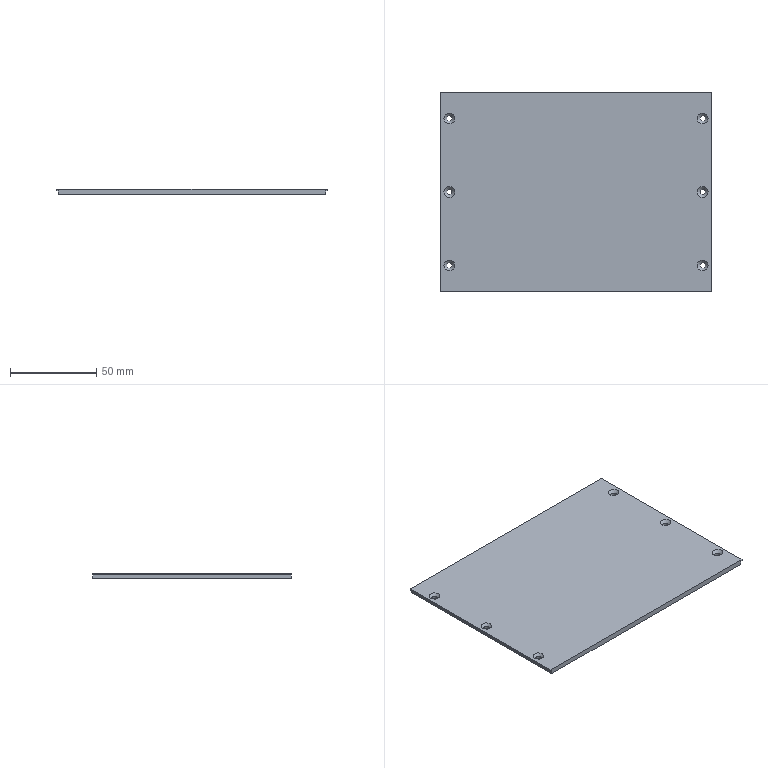Part | 1 solid | 50 faces | box 156.6 x 115 x 3 mm | volume 36735 mm3 | plane 26 | cylinder 18 | cone 6 | commonest cylinder face diameters 10 x12 3.2 x6
STEP:
#1=CARTESIAN_POINT('',(0.,115.,3.));
#2=VERTEX_POINT('',#1);
#3=CARTESIAN_POINT('',(0.,115.,2.1));
#4=VERTEX_POINT('',#3);
#5=CARTESIAN_POINT('',(0.,115.,3.));
#6=DIRECTION('',(0.,0.,-1.));
#7=VECTOR('',#6,1000.);
#8=LINE('',#5,#7);
#9=EDGE_CURVE('',#2,#4,#8,.T.);
#10=ORIENTED_EDGE('',*,*,#9,.T.);
#11=CARTESIAN_POINT('',(0.,0.,2.1));
#12=VERTEX_POINT('',#11);
#13=CARTESIAN_POINT('',(0.,-2.326,2.1));
#14=DIRECTION('',(0.,1.,0.));
#15=VECTOR('',#14,1000.);
#16=LINE('',#13,#15);
#17=EDGE_CURVE('',#12,#4,#16,.T.);
#18=ORIENTED_EDGE('',*,*,#17,.F.);
#19=CARTESIAN_POINT('',(0.,0.,3.));
#20=VERTEX_POINT('',#19);
#21=CARTESIAN_POINT('',(0.,0.,3.));
#22=DIRECTION('',(0.,0.,-1.));
#23=VECTOR('',#22,1000.);
#24=LINE('',#21,#23);
#25=EDGE_CURVE('',#20,#12,#24,.T.);
#26=ORIENTED_EDGE('',*,*,#25,.F.);
#27=CARTESIAN_POINT('',(0.,0.,3.));
#28=DIRECTION('',(0.,-1.,0.));
#29=VECTOR('',#28,1000.);
#30=LINE('',#27,#29);
#31=EDGE_CURVE('',#2,#20,#30,.T.);
#32=ORIENTED_EDGE('',*,*,#31,.F.);
#33=EDGE_LOOP('',(#10,#18,#26,#32));
#34=FACE_BOUND('',#33,.T.);
#35=CARTESIAN_POINT('',(0.,0.,3.));
#36=DIRECTION('',(1.,0.,0.));
#37=DIRECTION('',(0.,0.,-1.));
#38=AXIS2_PLACEMENT_3D('',#35,#36,#37);
#39=PLANE('',#38);
#40=ADVANCED_FACE('',(#34),#39,.F.);
#41=CARTESIAN_POINT('',(155.6,0.,2.1));
#42=VERTEX_POINT('',#41);
#43=CARTESIAN_POINT('',(155.6,0.,0.));
#44=VERTEX_POINT('',#43);
#45=CARTESIAN_POINT('',(155.6,0.,0.));
#46=DIRECTION('',(0.,0.,-1.));
#47=VECTOR('',#46,1000.);
#48=LINE('',#45,#47);
#49=EDGE_CURVE('',#42,#44,#48,.T.);
#50=ORIENTED_EDGE('',*,*,#49,.F.);
#51=CARTESIAN_POINT('',(156.6,0.,2.1));
#52=VERTEX_POINT('',#51);
#53=CARTESIAN_POINT('',(156.6,0.,2.1));
#54=DIRECTION('',(-1.,0.,0.));
#55=VECTOR('',#54,1000.);
#56=LINE('',#53,#55);
#57=EDGE_CURVE('',#52,#42,#56,.T.);
#58=ORIENTED_EDGE('',*,*,#57,.F.);
#59=CARTESIAN_POINT('',(156.6,0.,3.));
#60=VERTEX_POINT('',#59);
#61=CARTESIAN_POINT('',(156.6,0.,3.));
#62=DIRECTION('',(0.,0.,-1.));
#63=VECTOR('',#62,1000.);
#64=LINE('',#61,#63);
#65=EDGE_CURVE('',#60,#52,#64,.T.);
#66=ORIENTED_EDGE('',*,*,#65,.F.);
#67=CARTESIAN_POINT('',(0.,0.,3.));
#68=DIRECTION('',(1.,0.,0.));
#69=VECTOR('',#68,1000.);
#70=LINE('',#67,#69);
#71=EDGE_CURVE('',#20,#60,#70,.T.);
#72=ORIENTED_EDGE('',*,*,#71,.F.);
#73=ORIENTED_EDGE('',*,*,#25,.T.);
#74=CARTESIAN_POINT('',(1.,0.,2.1));
#75=VERTEX_POINT('',#74);
#76=CARTESIAN_POINT('',(0.,0.,2.1));
#77=DIRECTION('',(-1.,0.,0.));
#78=VECTOR('',#77,1000.);
#79=LINE('',#76,#78);
#80=EDGE_CURVE('',#75,#12,#79,.T.);
#81=ORIENTED_EDGE('',*,*,#80,.F.);
#82=CARTESIAN_POINT('',(1.,0.,0.));
#83=VERTEX_POINT('',#82);
#84=CARTESIAN_POINT('',(1.,0.,0.));
#85=DIRECTION('',(0.,0.,1.));
#86=VECTOR('',#85,1000.);
#87=LINE('',#84,#86);
#88=EDGE_CURVE('',#83,#75,#87,.T.);
#89=ORIENTED_EDGE('',*,*,#88,.F.);
#90=CARTESIAN_POINT('',(0.,0.,0.));
#91=DIRECTION('',(1.,0.,0.));
#92=VECTOR('',#91,1000.);
#93=LINE('',#90,#92);
#94=EDGE_CURVE('',#83,#44,#93,.T.);
#95=ORIENTED_EDGE('',*,*,#94,.T.);
#96=EDGE_LOOP('',(#50,#58,#66,#72,#73,#81,#89,#95));
#97=FACE_BOUND('',#96,.T.);
#98=CARTESIAN_POINT('',(0.,0.,3.));
#99=DIRECTION('',(0.,1.,0.));
#100=DIRECTION('',(0.,0.,1.));
#101=AXIS2_PLACEMENT_3D('',#98,#99,#100);
#102=PLANE('',#101);
#103=ADVANCED_FACE('',(#97),#102,.F.);
#104=ORIENTED_EDGE('',*,*,#65,.T.);
#105=CARTESIAN_POINT('',(156.6,115.,2.1));
#106=VERTEX_POINT('',#105);
#107=CARTESIAN_POINT('',(156.6,-2.326,2.1));
#108=DIRECTION('',(0.,1.,0.));
#109=VECTOR('',#108,1000.);
#110=LINE('',#107,#109);
#111=EDGE_CURVE('',#52,#106,#110,.T.);
#112=ORIENTED_EDGE('',*,*,#111,.T.);
#113=CARTESIAN_POINT('',(156.6,115.,3.));
#114=VERTEX_POINT('',#113);
#115=CARTESIAN_POINT('',(156.6,115.,3.));
#116=DIRECTION('',(0.,0.,-1.));
#117=VECTOR('',#116,1000.);
#118=LINE('',#115,#117);
#119=EDGE_CURVE('',#114,#106,#118,.T.);
#120=ORIENTED_EDGE('',*,*,#119,.F.);
#121=CARTESIAN_POINT('',(156.6,0.,3.));
#122=DIRECTION('',(0.,1.,0.));
#123=VECTOR('',#122,1000.);
#124=LINE('',#121,#123);
#125=EDGE_CURVE('',#60,#114,#124,.T.);
#126=ORIENTED_EDGE('',*,*,#125,.F.);
#127=EDGE_LOOP('',(#104,#112,#120,#126));
#128=FACE_BOUND('',#127,.T.);
#129=CARTESIAN_POINT('',(156.6,0.,3.));
#130=DIRECTION('',(-1.,0.,0.));
#131=DIRECTION('',(0.,0.,1.));
#132=AXIS2_PLACEMENT_3D('',#129,#130,#131);
#133=PLANE('',#132);
#134=ADVANCED_FACE('',(#128),#133,.F.);
#135=ORIENTED_EDGE('',*,*,#119,.T.);
#136=CARTESIAN_POINT('',(155.6,115.,2.1));
#137=VERTEX_POINT('',#136);
#138=CARTESIAN_POINT('',(156.6,115.,2.1));
#139=DIRECTION('',(1.,0.,0.));
#140=VECTOR('',#139,1000.);
#141=LINE('',#138,#140);
#142=EDGE_CURVE('',#137,#106,#141,.T.);
#143=ORIENTED_EDGE('',*,*,#142,.F.);
#144=CARTESIAN_POINT('',(155.6,115.,0.));
#145=VERTEX_POINT('',#144);
#146=CARTESIAN_POINT('',(155.6,115.,0.));
#147=DIRECTION('',(0.,0.,1.));
#148=VECTOR('',#147,1000.);
#149=LINE('',#146,#148);
#150=EDGE_CURVE('',#145,#137,#149,.T.);
#151=ORIENTED_EDGE('',*,*,#150,.F.);
#152=CARTESIAN_POINT('',(1.,115.,0.));
#153=VERTEX_POINT('',#152);
#154=CARTESIAN_POINT('',(0.,115.,0.));
#155=DIRECTION('',(-1.,0.,0.));
#156=VECTOR('',#155,1000.);
#157=LINE('',#154,#156);
#158=EDGE_CURVE('',#145,#153,#157,.T.);
#159=ORIENTED_EDGE('',*,*,#158,.T.);
#160=CARTESIAN_POINT('',(1.,115.,2.1));
#161=VERTEX_POINT('',#160);
#162=CARTESIAN_POINT('',(1.,115.,0.));
#163=DIRECTION('',(0.,0.,-1.));
#164=VECTOR('',#163,1000.);
#165=LINE('',#162,#164);
#166=EDGE_CURVE('',#161,#153,#165,.T.);
#167=ORIENTED_EDGE('',*,*,#166,.F.);
#168=CARTESIAN_POINT('',(0.,115.,2.1));
#169=DIRECTION('',(1.,0.,0.));
#170=VECTOR('',#169,1000.);
#171=LINE('',#168,#170);
#172=EDGE_CURVE('',#4,#161,#171,.T.);
#173=ORIENTED_EDGE('',*,*,#172,.F.);
#174=ORIENTED_EDGE('',*,*,#9,.F.);
#175=CARTESIAN_POINT('',(0.,115.,3.));
#176=DIRECTION('',(-1.,0.,0.));
#177=VECTOR('',#176,1000.);
#178=LINE('',#175,#177);
#179=EDGE_CURVE('',#114,#2,#178,.T.);
#180=ORIENTED_EDGE('',*,*,#179,.F.);
#181=EDGE_LOOP('',(#135,#143,#151,#159,#167,#173,#174,#180));
#182=FACE_BOUND('',#181,.T.);
#183=CARTESIAN_POINT('',(0.,115.,3.));
#184=DIRECTION('',(0.,-1.,0.));
#185=DIRECTION('',(0.,0.,-1.));
#186=AXIS2_PLACEMENT_3D('',#183,#184,#185);
#187=PLANE('',#186);
#188=ADVANCED_FACE('',(#182),#187,.F.);
#189=CARTESIAN_POINT('',(148.5,15.,3.));
#190=VERTEX_POINT('',#189);
#191=CARTESIAN_POINT('',(151.6,15.,3.));
#192=DIRECTION('',(0.,0.,-1.));
#193=DIRECTION('',(-1.,0.,0.));
#194=AXIS2_PLACEMENT_3D('',#191,#192,#193);
#195=CIRCLE('',#194,3.1);
#196=EDGE_CURVE('',#190,#190,#195,.T.);
#197=ORIENTED_EDGE('',*,*,#196,.T.);
#198=EDGE_LOOP('',(#197));
#199=FACE_BOUND('',#198,.T.);
#200=CARTESIAN_POINT('',(148.5,57.5,3.));
#201=VERTEX_POINT('',#200);
#202=CARTESIAN_POINT('',(151.6,57.5,3.));
#203=DIRECTION('',(0.,0.,-1.));
#204=DIRECTION('',(-1.,0.,0.));
#205=AXIS2_PLACEMENT_3D('',#202,#203,#204);
#206=CIRCLE('',#205,3.1);
#207=EDGE_CURVE('',#201,#201,#206,.T.);
#208=ORIENTED_EDGE('',*,*,#207,.T.);
#209=EDGE_LOOP('',(#208));
#210=FACE_BOUND('',#209,.T.);
#211=CARTESIAN_POINT('',(148.5,100.,3.));
#212=VERTEX_POINT('',#211);
#213=CARTESIAN_POINT('',(151.6,100.,3.));
#214=DIRECTION('',(0.,0.,-1.));
#215=DIRECTION('',(-1.,0.,0.));
#216=AXIS2_PLACEMENT_3D('',#213,#214,#215);
#217=CIRCLE('',#216,3.1);
#218=EDGE_CURVE('',#212,#212,#217,.T.);
#219=ORIENTED_EDGE('',*,*,#218,.T.);
#220=EDGE_LOOP('',(#219));
#221=FACE_BOUND('',#220,.T.);
#222=CARTESIAN_POINT('',(1.9,15.,3.));
#223=VERTEX_POINT('',#222);
#224=CARTESIAN_POINT('',(5.,15.,3.));
#225=DIRECTION('',(0.,0.,-1.));
#226=DIRECTION('',(-1.,0.,0.));
#227=AXIS2_PLACEMENT_3D('',#224,#225,#226);
#228=CIRCLE('',#227,3.1);
#229=EDGE_CURVE('',#223,#223,#228,.T.);
#230=ORIENTED_EDGE('',*,*,#229,.T.);
#231=EDGE_LOOP('',(#230));
#232=FACE_BOUND('',#231,.T.);
#233=CARTESIAN_POINT('',(1.9,57.5,3.));
#234=VERTEX_POINT('',#233);
#235=CARTESIAN_POINT('',(5.,57.5,3.));
#236=DIRECTION('',(0.,0.,-1.));
#237=DIRECTION('',(-1.,0.,0.));
#238=AXIS2_PLACEMENT_3D('',#235,#236,#237);
#239=CIRCLE('',#238,3.1);
#240=EDGE_CURVE('',#234,#234,#239,.T.);
#241=ORIENTED_EDGE('',*,*,#240,.T.);
#242=EDGE_LOOP('',(#241));
#243=FACE_BOUND('',#242,.T.);
#244=CARTESIAN_POINT('',(1.9,100.,3.));
#245=VERTEX_POINT('',#244);
#246=CARTESIAN_POINT('',(5.,100.,3.));
#247=DIRECTION('',(0.,0.,-1.));
#248=DIRECTION('',(-1.,0.,0.));
#249=AXIS2_PLACEMENT_3D('',#246,#247,#248);
#250=CIRCLE('',#249,3.1);
#251=EDGE_CURVE('',#245,#245,#250,.T.);
#252=ORIENTED_EDGE('',*,*,#251,.T.);
#253=EDGE_LOOP('',(#252));
#254=FACE_BOUND('',#253,.T.);
#255=ORIENTED_EDGE('',*,*,#31,.T.);
#256=ORIENTED_EDGE('',*,*,#71,.T.);
#257=ORIENTED_EDGE('',*,*,#125,.T.);
#258=ORIENTED_EDGE('',*,*,#179,.T.);
#259=EDGE_LOOP('',(#255,#256,#257,#258));
#260=FACE_BOUND('',#259,.T.);
#261=CARTESIAN_POINT('',(0.,0.,3.));
#262=DIRECTION('',(0.,0.,-1.));
#263=DIRECTION('',(-1.,0.,0.));
#264=AXIS2_PLACEMENT_3D('',#261,#262,#263);
#265=PLANE('',#264);
#266=ADVANCED_FACE('',(#199,#210,#221,#232,#243,#254,#260),#265,.F.);
#267=CARTESIAN_POINT('',(81.083,52.031,0.));
#268=VERTEX_POINT('',#267);
#269=CARTESIAN_POINT('',(130.154,19.154,0.));
#270=VERTEX_POINT('',#269);
#271=CARTESIAN_POINT('',(78.3,53.896,0.));
#272=DIRECTION('',(0.8308,-0.5566,0.));
#273=VECTOR('',#272,1000.);
#274=LINE('',#271,#273);
#275=EDGE_CURVE('',#268,#270,#274,.T.);
#276=ORIENTED_EDGE('',*,*,#275,.F.);
#277=CARTESIAN_POINT('',(75.517,52.031,0.));
#278=VERTEX_POINT('',#277);
#279=CARTESIAN_POINT('',(78.3,47.878,0.));
#280=DIRECTION('',(0.,0.,-1.));
#281=DIRECTION('',(-1.,0.,0.));
#282=AXIS2_PLACEMENT_3D('',#279,#280,#281);
#283=CIRCLE('',#282,5.);
#284=EDGE_CURVE('',#268,#278,#283,.F.);
#285=ORIENTED_EDGE('',*,*,#284,.T.);
#286=CARTESIAN_POINT('',(26.446,19.154,0.));
#287=VERTEX_POINT('',#286);
#288=CARTESIAN_POINT('',(78.3,53.896,0.));
#289=DIRECTION('',(0.8308,0.5566,0.));
#290=VECTOR('',#289,1000.);
#291=LINE('',#288,#290);
#292=EDGE_CURVE('',#287,#278,#291,.T.);
#293=ORIENTED_EDGE('',*,*,#292,.F.);
#294=CARTESIAN_POINT('',(29.229,10.,0.));
#295=VERTEX_POINT('',#294);
#296=CARTESIAN_POINT('',(29.229,15.,0.));
#297=DIRECTION('',(0.,0.,-1.));
#298=DIRECTION('',(-1.,0.,0.));
#299=AXIS2_PLACEMENT_3D('',#296,#297,#298);
#300=CIRCLE('',#299,5.);
#301=EDGE_CURVE('',#287,#295,#300,.F.);
#302=ORIENTED_EDGE('',*,*,#301,.T.);
#303=CARTESIAN_POINT('',(127.371,10.,0.));
#304=VERTEX_POINT('',#303);
#305=CARTESIAN_POINT('',(143.817,10.,0.));
#306=DIRECTION('',(-1.,0.,0.));
#307=VECTOR('',#306,1000.);
#308=LINE('',#305,#307);
#309=EDGE_CURVE('',#304,#295,#308,.T.);
#310=ORIENTED_EDGE('',*,*,#309,.F.);
#311=CARTESIAN_POINT('',(127.371,15.,0.));
#312=DIRECTION('',(0.,0.,-1.));
#313=DIRECTION('',(-1.,0.,0.));
#314=AXIS2_PLACEMENT_3D('',#311,#312,#313);
#315=CIRCLE('',#314,5.);
#316=EDGE_CURVE('',#304,#270,#315,.F.);
#317=ORIENTED_EDGE('',*,*,#316,.T.);
#318=EDGE_LOOP('',(#276,#285,#293,#302,#310,#317));
#319=FACE_BOUND('',#318,.T.);
#320=CARTESIAN_POINT('',(10.,23.522,0.));
#321=VERTEX_POINT('',#320);
#322=CARTESIAN_POINT('',(10.,91.478,0.));
#323=VERTEX_POINT('',#322);
#324=CARTESIAN_POINT('',(10.,14.154,0.));
#325=DIRECTION('',(0.,1.,0.));
#326=VECTOR('',#325,1000.);
#327=LINE('',#324,#326);
#328=EDGE_CURVE('',#321,#323,#327,.T.);
#329=ORIENTED_EDGE('',*,*,#328,.F.);
#330=CARTESIAN_POINT('',(17.783,19.368,0.));
#331=VERTEX_POINT('',#330);
#332=CARTESIAN_POINT('',(15.,23.522,0.));
#333=DIRECTION('',(0.,0.,-1.));
#334=DIRECTION('',(-1.,0.,0.));
#335=AXIS2_PLACEMENT_3D('',#332,#333,#334);
#336=CIRCLE('',#335,5.);
#337=EDGE_CURVE('',#321,#331,#336,.F.);
#338=ORIENTED_EDGE('',*,*,#337,.T.);
#339=CARTESIAN_POINT('',(68.496,53.346,0.));
#340=VERTEX_POINT('',#339);
#341=CARTESIAN_POINT('',(10.,14.154,0.));
#342=DIRECTION('',(-0.8308,-0.5566,0.));
#343=VECTOR('',#342,1000.);
#344=LINE('',#341,#343);
#345=EDGE_CURVE('',#340,#331,#344,.T.);
#346=ORIENTED_EDGE('',*,*,#345,.F.);
#347=CARTESIAN_POINT('',(68.496,61.654,0.));
#348=VERTEX_POINT('',#347);
#349=CARTESIAN_POINT('',(65.713,57.5,0.));
#350=DIRECTION('',(0.,0.,-1.));
#351=DIRECTION('',(-1.,0.,0.));
#352=AXIS2_PLACEMENT_3D('',#349,#350,#351);
#353=CIRCLE('',#352,5.);
#354=EDGE_CURVE('',#340,#348,#353,.F.);
#355=ORIENTED_EDGE('',*,*,#354,.T.);
#356=CARTESIAN_POINT('',(17.783,95.632,0.));
#357=VERTEX_POINT('',#356);
#358=CARTESIAN_POINT('',(10.,100.846,0.));
#359=DIRECTION('',(0.8308,-0.5566,0.));
#360=VECTOR('',#359,1000.);
#361=LINE('',#358,#360);
#362=EDGE_CURVE('',#357,#348,#361,.T.);
#363=ORIENTED_EDGE('',*,*,#362,.F.);
#364=CARTESIAN_POINT('',(15.,91.478,0.));
#365=DIRECTION('',(0.,0.,-1.));
#366=DIRECTION('',(-1.,0.,0.));
#367=AXIS2_PLACEMENT_3D('',#364,#365,#366);
#368=CIRCLE('',#367,5.);
#369=EDGE_CURVE('',#357,#323,#368,.F.);
#370=ORIENTED_EDGE('',*,*,#369,.T.);
#371=EDGE_LOOP('',(#329,#338,#346,#355,#363,#370));
#372=FACE_BOUND('',#371,.T.);
#373=CARTESIAN_POINT('',(75.517,62.969,0.));
#374=VERTEX_POINT('',#373);
#375=CARTESIAN_POINT('',(26.446,95.846,0.));
#376=VERTEX_POINT('',#375);
#377=CARTESIAN_POINT('',(78.3,61.104,0.));
#378=DIRECTION('',(-0.8308,0.5566,0.));
#379=VECTOR('',#378,1000.);
#380=LINE('',#377,#379);
#381=EDGE_CURVE('',#374,#376,#380,.T.);
#382=ORIENTED_EDGE('',*,*,#381,.F.);
#383=CARTESIAN_POINT('',(81.083,62.969,0.));
#384=VERTEX_POINT('',#383);
#385=CARTESIAN_POINT('',(78.3,67.122,0.));
#386=DIRECTION('',(0.,0.,-1.));
#387=DIRECTION('',(-1.,0.,0.));
#388=AXIS2_PLACEMENT_3D('',#385,#386,#387);
#389=CIRCLE('',#388,5.);
#390=EDGE_CURVE('',#374,#384,#389,.F.);
#391=ORIENTED_EDGE('',*,*,#390,.T.);
#392=CARTESIAN_POINT('',(130.154,95.846,0.));
#393=VERTEX_POINT('',#392);
#394=CARTESIAN_POINT('',(78.3,61.104,0.));
#395=DIRECTION('',(-0.8308,-0.5566,0.));
#396=VECTOR('',#395,1000.);
#397=LINE('',#394,#396);
#398=EDGE_CURVE('',#393,#384,#397,.T.);
#399=ORIENTED_EDGE('',*,*,#398,.F.);
#400=CARTESIAN_POINT('',(127.371,105.,0.));
#401=VERTEX_POINT('',#400);
#402=CARTESIAN_POINT('',(127.371,100.,0.));
#403=DIRECTION('',(0.,0.,-1.));
#404=DIRECTION('',(-1.,0.,0.));
#405=AXIS2_PLACEMENT_3D('',#402,#403,#404);
#406=CIRCLE('',#405,5.);
#407=EDGE_CURVE('',#393,#401,#406,.F.);
#408=ORIENTED_EDGE('',*,*,#407,.T.);
#409=CARTESIAN_POINT('',(29.229,105.,0.));
#410=VERTEX_POINT('',#409);
#411=CARTESIAN_POINT('',(143.817,105.,0.));
#412=DIRECTION('',(1.,0.,0.));
#413=VECTOR('',#412,1000.);
#414=LINE('',#411,#413);
#415=EDGE_CURVE('',#410,#401,#414,.T.);
#416=ORIENTED_EDGE('',*,*,#415,.F.);
#417=CARTESIAN_POINT('',(29.229,100.,0.));
#418=DIRECTION('',(0.,0.,-1.));
#419=DIRECTION('',(-1.,0.,0.));
#420=AXIS2_PLACEMENT_3D('',#417,#418,#419);
#421=CIRCLE('',#420,5.);
#422=EDGE_CURVE('',#410,#376,#421,.F.);
#423=ORIENTED_EDGE('',*,*,#422,.T.);
#424=EDGE_LOOP('',(#382,#391,#399,#408,#416,#423));
#425=FACE_BOUND('',#424,.T.);
#426=CARTESIAN_POINT('',(88.104,61.654,0.));
#427=VERTEX_POINT('',#426);
#428=CARTESIAN_POINT('',(138.817,95.632,0.));
#429=VERTEX_POINT('',#428);
#430=CARTESIAN_POINT('',(146.6,100.846,0.));
#431=DIRECTION('',(0.8308,0.5566,0.));
#432=VECTOR('',#431,1000.);
#433=LINE('',#430,#432);
#434=EDGE_CURVE('',#427,#429,#433,.T.);
#435=ORIENTED_EDGE('',*,*,#434,.F.);
#436=CARTESIAN_POINT('',(88.104,53.346,0.));
#437=VERTEX_POINT('',#436);
#438=CARTESIAN_POINT('',(90.887,57.5,0.));
#439=DIRECTION('',(0.,0.,-1.));
#440=DIRECTION('',(-1.,0.,0.));
#441=AXIS2_PLACEMENT_3D('',#438,#439,#440);
#442=CIRCLE('',#441,5.);
#443=EDGE_CURVE('',#427,#437,#442,.F.);
#444=ORIENTED_EDGE('',*,*,#443,.T.);
#445=CARTESIAN_POINT('',(138.817,19.368,0.));
#446=VERTEX_POINT('',#445);
#447=CARTESIAN_POINT('',(146.6,14.154,0.));
#448=DIRECTION('',(-0.8308,0.5566,0.));
#449=VECTOR('',#448,1000.);
#450=LINE('',#447,#449);
#451=EDGE_CURVE('',#446,#437,#450,.T.);
#452=ORIENTED_EDGE('',*,*,#451,.F.);
#453=CARTESIAN_POINT('',(146.6,23.522,0.));
#454=VERTEX_POINT('',#453);
#455=CARTESIAN_POINT('',(141.6,23.522,0.));
#456=DIRECTION('',(0.,0.,-1.));
#457=DIRECTION('',(-1.,0.,0.));
#458=AXIS2_PLACEMENT_3D('',#455,#456,#457);
#459=CIRCLE('',#458,5.);
#460=EDGE_CURVE('',#446,#454,#459,.F.);
#461=ORIENTED_EDGE('',*,*,#460,.T.);
#462=CARTESIAN_POINT('',(146.6,91.478,0.));
#463=VERTEX_POINT('',#462);
#464=CARTESIAN_POINT('',(146.6,14.154,0.));
#465=DIRECTION('',(0.,-1.,0.));
#466=VECTOR('',#465,1000.);
#467=LINE('',#464,#466);
#468=EDGE_CURVE('',#463,#454,#467,.T.);
#469=ORIENTED_EDGE('',*,*,#468,.F.);
#470=CARTESIAN_POINT('',(141.6,91.478,0.));
#471=DIRECTION('',(0.,0.,-1.));
#472=DIRECTION('',(-1.,0.,0.));
#473=AXIS2_PLACEMENT_3D('',#470,#471,#472);
#474=CIRCLE('',#473,5.);
#475=EDGE_CURVE('',#463,#429,#474,.F.);
#476=ORIENTED_EDGE('',*,*,#475,.T.);
#477=EDGE_LOOP('',(#435,#444,#452,#461,#469,#476));
#478=FACE_BOUND('',#477,.T.);
#479=CARTESIAN_POINT('',(155.6,-2.326,0.));
#480=DIRECTION('',(0.,1.,0.));
#481=VECTOR('',#480,1000.);
#482=LINE('',#479,#481);
#483=EDGE_CURVE('',#44,#145,#482,.T.);
#484=ORIENTED_EDGE('',*,*,#483,.F.);
#485=ORIENTED_EDGE('',*,*,#94,.F.);
#486=CARTESIAN_POINT('',(1.,-2.326,0.));
#487=DIRECTION('',(0.,1.,0.));
#488=VECTOR('',#487,1000.);
#489=LINE('',#486,#488);
#490=EDGE_CURVE('',#83,#153,#489,.T.);
#491=ORIENTED_EDGE('',*,*,#490,.T.);
#492=ORIENTED_EDGE('',*,*,#158,.F.);
#493=EDGE_LOOP('',(#484,#485,#491,#492));
#494=FACE_BOUND('',#493,.T.);
#495=CARTESIAN_POINT('',(150.,100.,0.));
#496=VERTEX_POINT('',#495);
#497=CARTESIAN_POINT('',(151.6,100.,0.));
#498=DIRECTION('',(0.,0.,-1.));
#499=DIRECTION('',(-1.,0.,0.));
#500=AXIS2_PLACEMENT_3D('',#497,#498,#499);
#501=CIRCLE('',#500,1.6);
#502=EDGE_CURVE('',#496,#496,#501,.F.);
#503=ORIENTED_EDGE('',*,*,#502,.T.);
#504=EDGE_LOOP('',(#503));
#505=FACE_BOUND('',#504,.T.);
#506=CARTESIAN_POINT('',(150.,57.5,0.));
#507=VERTEX_POINT('',#506);
#508=CARTESIAN_POINT('',(151.6,57.5,0.));
#509=DIRECTION('',(0.,0.,-1.));
#510=DIRECTION('',(-1.,0.,0.));
#511=AXIS2_PLACEMENT_3D('',#508,#509,#510);
#512=CIRCLE('',#511,1.6);
#513=EDGE_CURVE('',#507,#507,#512,.F.);
#514=ORIENTED_EDGE('',*,*,#513,.T.);
#515=EDGE_LOOP('',(#514));
#516=FACE_BOUND('',#515,.T.);
#517=CARTESIAN_POINT('',(150.,15.,0.));
#518=VERTEX_POINT('',#517);
#519=CARTESIAN_POINT('',(151.6,15.,0.));
#520=DIRECTION('',(0.,0.,-1.));
#521=DIRECTION('',(-1.,0.,0.));
#522=AXIS2_PLACEMENT_3D('',#519,#520,#521);
#523=CIRCLE('',#522,1.6);
#524=EDGE_CURVE('',#518,#518,#523,.F.);
#525=ORIENTED_EDGE('',*,*,#524,.T.);
#526=EDGE_LOOP('',(#525));
#527=FACE_BOUND('',#526,.T.);
#528=CARTESIAN_POINT('',(3.4,15.,0.));
#529=VERTEX_POINT('',#528);
#530=CARTESIAN_POINT('',(5.,15.,0.));
#531=DIRECTION('',(0.,0.,-1.));
#532=DIRECTION('',(-1.,0.,0.));
#533=AXIS2_PLACEMENT_3D('',#530,#531,#532);
#534=CIRCLE('',#533,1.6);
#535=EDGE_CURVE('',#529,#529,#534,.F.);
#536=ORIENTED_EDGE('',*,*,#535,.T.);
#537=EDGE_LOOP('',(#536));
#538=FACE_BOUND('',#537,.T.);
#539=CARTESIAN_POINT('',(3.4,57.5,0.));
#540=VERTEX_POINT('',#539);
#541=CARTESIAN_POINT('',(5.,57.5,0.));
#542=DIRECTION('',(0.,0.,-1.));
#543=DIRECTION('',(-1.,0.,0.));
#544=AXIS2_PLACEMENT_3D('',#541,#542,#543);
#545=CIRCLE('',#544,1.6);
#546=EDGE_CURVE('',#540,#540,#545,.F.);
#547=ORIENTED_EDGE('',*,*,#546,.T.);
#548=EDGE_LOOP('',(#547));
#549=FACE_BOUND('',#548,.T.);
#550=CARTESIAN_POINT('',(3.4,100.,0.));
#551=VERTEX_POINT('',#550);
#552=CARTESIAN_POINT('',(5.,100.,0.));
#553=DIRECTION('',(0.,0.,-1.));
#554=DIRECTION('',(-1.,0.,0.));
#555=AXIS2_PLACEMENT_3D('',#552,#553,#554);
#556=CIRCLE('',#555,1.6);
#557=EDGE_CURVE('',#551,#551,#556,.F.);
#558=ORIENTED_EDGE('',*,*,#557,.T.);
#559=EDGE_LOOP('',(#558));
#560=FACE_BOUND('',#559,.T.);
#561=CARTESIAN_POINT('',(0.,0.,0.));
#562=DIRECTION('',(0.,0.,-1.));
#563=DIRECTION('',(-1.,0.,0.));
#564=AXIS2_PLACEMENT_3D('',#561,#562,#563);
#565=PLANE('',#564);
#566=ADVANCED_FACE('',(#319,#372,#425,#478,#494,#505,#516,#527,#538,#549,#560),#565,.T.);
#567=CARTESIAN_POINT('',(3.4,100.,1.5));
#568=VERTEX_POINT('',#567);
#569=CARTESIAN_POINT('',(5.,100.,1.5));
#570=DIRECTION('',(0.,0.,-1.));
#571=DIRECTION('',(-1.,0.,0.));
#572=AXIS2_PLACEMENT_3D('',#569,#570,#571);
#573=CIRCLE('',#572,1.6);
#574=EDGE_CURVE('',#568,#568,#573,.F.);
#575=ORIENTED_EDGE('',*,*,#574,.T.);
#576=EDGE_LOOP('',(#575));
#577=FACE_BOUND('',#576,.T.);
#578=ORIENTED_EDGE('',*,*,#557,.F.);
#579=EDGE_LOOP('',(#578));
#580=FACE_BOUND('',#579,.T.);
#581=CARTESIAN_POINT('',(5.,100.,-4.525));
#582=DIRECTION('',(0.,0.,1.));
#583=DIRECTION('',(1.,0.,0.));
#584=AXIS2_PLACEMENT_3D('',#581,#582,#583);
#585=CYLINDRICAL_SURFACE('',#584,1.6);
#586=ADVANCED_FACE('',(#577,#580),#585,.F.);
#587=CARTESIAN_POINT('',(3.4,57.5,1.5));
#588=VERTEX_POINT('',#587);
#589=CARTESIAN_POINT('',(5.,57.5,1.5));
#590=DIRECTION('',(0.,0.,-1.));
#591=DIRECTION('',(-1.,0.,0.));
#592=AXIS2_PLACEMENT_3D('',#589,#590,#591);
#593=CIRCLE('',#592,1.6);
#594=EDGE_CURVE('',#588,#588,#593,.F.);
#595=ORIENTED_EDGE('',*,*,#594,.T.);
#596=EDGE_LOOP('',(#595));
#597=FACE_BOUND('',#596,.T.);
#598=ORIENTED_EDGE('',*,*,#546,.F.);
#599=EDGE_LOOP('',(#598));
#600=FACE_BOUND('',#599,.T.);
#601=CARTESIAN_POINT('',(5.,57.5,-4.525));
#602=DIRECTION('',(0.,0.,1.));
#603=DIRECTION('',(1.,0.,0.));
#604=AXIS2_PLACEMENT_3D('',#601,#602,#603);
#605=CYLINDRICAL_SURFACE('',#604,1.6);
#606=ADVANCED_FACE('',(#597,#600),#605,.F.);
#607=CARTESIAN_POINT('',(3.4,15.,1.5));
#608=VERTEX_POINT('',#607);
#609=CARTESIAN_POINT('',(5.,15.,1.5));
#610=DIRECTION('',(0.,0.,-1.));
#611=DIRECTION('',(-1.,0.,0.));
#612=AXIS2_PLACEMENT_3D('',#609,#610,#611);
#613=CIRCLE('',#612,1.6);
#614=EDGE_CURVE('',#608,#608,#613,.F.);
#615=ORIENTED_EDGE('',*,*,#614,.T.);
#616=EDGE_LOOP('',(#615));
#617=FACE_BOUND('',#616,.T.);
#618=ORIENTED_EDGE('',*,*,#535,.F.);
#619=EDGE_LOOP('',(#618));
#620=FACE_BOUND('',#619,.T.);
#621=CARTESIAN_POINT('',(5.,15.,-4.525));
#622=DIRECTION('',(0.,0.,1.));
#623=DIRECTION('',(1.,0.,0.));
#624=AXIS2_PLACEMENT_3D('',#621,#622,#623);
#625=CYLINDRICAL_SURFACE('',#624,1.6);
#626=ADVANCED_FACE('',(#617,#620),#625,.F.);
#627=CARTESIAN_POINT('',(150.,15.,1.5));
#628=VERTEX_POINT('',#627);
#629=CARTESIAN_POINT('',(151.6,15.,1.5));
#630=DIRECTION('',(0.,0.,-1.));
#631=DIRECTION('',(-1.,0.,0.));
#632=AXIS2_PLACEMENT_3D('',#629,#630,#631);
#633=CIRCLE('',#632,1.6);
#634=EDGE_CURVE('',#628,#628,#633,.F.);
#635=ORIENTED_EDGE('',*,*,#634,.T.);
#636=EDGE_LOOP('',(#635));
#637=FACE_BOUND('',#636,.T.);
#638=ORIENTED_EDGE('',*,*,#524,.F.);
#639=EDGE_LOOP('',(#638));
#640=FACE_BOUND('',#639,.T.);
#641=CARTESIAN_POINT('',(151.6,15.,-4.525));
#642=DIRECTION('',(0.,0.,1.));
#643=DIRECTION('',(1.,0.,0.));
#644=AXIS2_PLACEMENT_3D('',#641,#642,#643);
#645=CYLINDRICAL_SURFACE('',#644,1.6);
#646=ADVANCED_FACE('',(#637,#640),#645,.F.);
#647=CARTESIAN_POINT('',(150.,57.5,1.5));
#648=VERTEX_POINT('',#647);
#649=CARTESIAN_POINT('',(151.6,57.5,1.5));
#650=DIRECTION('',(0.,0.,-1.));
#651=DIRECTION('',(-1.,0.,0.));
#652=AXIS2_PLACEMENT_3D('',#649,#650,#651);
#653=CIRCLE('',#652,1.6);
#654=EDGE_CURVE('',#648,#648,#653,.F.);
#655=ORIENTED_EDGE('',*,*,#654,.T.);
#656=EDGE_LOOP('',(#655));
#657=FACE_BOUND('',#656,.T.);
#658=ORIENTED_EDGE('',*,*,#513,.F.);
#659=EDGE_LOOP('',(#658));
#660=FACE_BOUND('',#659,.T.);
#661=CARTESIAN_POINT('',(151.6,57.5,-4.525));
#662=DIRECTION('',(0.,0.,1.));
#663=DIRECTION('',(1.,0.,0.));
#664=AXIS2_PLACEMENT_3D('',#661,#662,#663);
#665=CYLINDRICAL_SURFACE('',#664,1.6);
#666=ADVANCED_FACE('',(#657,#660),#665,.F.);
#667=CARTESIAN_POINT('',(150.,100.,1.5));
#668=VERTEX_POINT('',#667);
#669=CARTESIAN_POINT('',(151.6,100.,1.5));
#670=DIRECTION('',(0.,0.,-1.));
#671=DIRECTION('',(-1.,0.,0.));
#672=AXIS2_PLACEMENT_3D('',#669,#670,#671);
#673=CIRCLE('',#672,1.6);
#674=EDGE_CURVE('',#668,#668,#673,.F.);
#675=ORIENTED_EDGE('',*,*,#674,.T.);
#676=EDGE_LOOP('',(#675));
#677=FACE_BOUND('',#676,.T.);
#678=ORIENTED_EDGE('',*,*,#502,.F.);
#679=EDGE_LOOP('',(#678));
#680=FACE_BOUND('',#679,.T.);
#681=CARTESIAN_POINT('',(151.6,100.,-4.525));
#682=DIRECTION('',(0.,0.,1.));
#683=DIRECTION('',(1.,0.,0.));
#684=AXIS2_PLACEMENT_3D('',#681,#682,#683);
#685=CYLINDRICAL_SURFACE('',#684,1.6);
#686=ADVANCED_FACE('',(#677,#680),#685,.F.);
#687=ORIENTED_EDGE('',*,*,#88,.T.);
#688=CARTESIAN_POINT('',(1.,-2.326,2.1));
#689=DIRECTION('',(0.,1.,0.));
#690=VECTOR('',#689,1000.);
#691=LINE('',#688,#690);
#692=EDGE_CURVE('',#75,#161,#691,.T.);
#693=ORIENTED_EDGE('',*,*,#692,.T.);
#694=ORIENTED_EDGE('',*,*,#166,.T.);
#695=ORIENTED_EDGE('',*,*,#490,.F.);
#696=EDGE_LOOP('',(#687,#693,#694,#695));
#697=FACE_BOUND('',#696,.T.);
#698=CARTESIAN_POINT('',(1.,-2.326,0.));
#699=DIRECTION('',(1.,0.,0.));
#700=DIRECTION('',(0.,0.,-1.));
#701=AXIS2_PLACEMENT_3D('',#698,#699,#700);
#702=PLANE('',#701);
#703=ADVANCED_FACE('',(#697),#702,.F.);
#704=ORIENTED_EDGE('',*,*,#80,.T.);
#705=ORIENTED_EDGE('',*,*,#17,.T.);
#706=ORIENTED_EDGE('',*,*,#172,.T.);
#707=ORIENTED_EDGE('',*,*,#692,.F.);
#708=EDGE_LOOP('',(#704,#705,#706,#707));
#709=FACE_BOUND('',#708,.T.);
#710=CARTESIAN_POINT('',(0.,-2.326,2.1));
#711=DIRECTION('',(0.,0.,1.));
#712=DIRECTION('',(1.,0.,0.));
#713=AXIS2_PLACEMENT_3D('',#710,#711,#712);
#714=PLANE('',#713);
#715=ADVANCED_FACE('',(#709),#714,.F.);
#716=ORIENTED_EDGE('',*,*,#57,.T.);
#717=CARTESIAN_POINT('',(155.6,-2.326,2.1));
#718=DIRECTION('',(0.,1.,0.));
#719=VECTOR('',#718,1000.);
#720=LINE('',#717,#719);
#721=EDGE_CURVE('',#42,#137,#720,.T.);
#722=ORIENTED_EDGE('',*,*,#721,.T.);
#723=ORIENTED_EDGE('',*,*,#142,.T.);
#724=ORIENTED_EDGE('',*,*,#111,.F.);
#725=EDGE_LOOP('',(#716,#722,#723,#724));
#726=FACE_BOUND('',#725,.T.);
#727=CARTESIAN_POINT('',(156.6,-2.326,2.1));
#728=DIRECTION('',(0.,0.,1.));
#729=DIRECTION('',(1.,0.,0.));
#730=AXIS2_PLACEMENT_3D('',#727,#728,#729);
#731=PLANE('',#730);
#732=ADVANCED_FACE('',(#726),#731,.F.);
#733=ORIENTED_EDGE('',*,*,#49,.T.);
#734=ORIENTED_EDGE('',*,*,#483,.T.);
#735=ORIENTED_EDGE('',*,*,#150,.T.);
#736=ORIENTED_EDGE('',*,*,#721,.F.);
#737=EDGE_LOOP('',(#733,#734,#735,#736));
#738=FACE_BOUND('',#737,.T.);
#739=CARTESIAN_POINT('',(155.6,-2.326,0.));
#740=DIRECTION('',(-1.,0.,0.));
#741=DIRECTION('',(0.,0.,1.));
#742=AXIS2_PLACEMENT_3D('',#739,#740,#741);
#743=PLANE('',#742);
#744=ADVANCED_FACE('',(#738),#743,.F.);
#745=CARTESIAN_POINT('',(138.817,95.632,1.5));
#746=VERTEX_POINT('',#745);
#747=CARTESIAN_POINT('',(88.104,61.654,1.5));
#748=VERTEX_POINT('',#747);
#749=CARTESIAN_POINT('',(146.6,100.846,1.5));
#750=DIRECTION('',(-0.8308,-0.5566,0.));
#751=VECTOR('',#750,1000.);
#752=LINE('',#749,#751);
#753=EDGE_CURVE('',#746,#748,#752,.T.);
#754=ORIENTED_EDGE('',*,*,#753,.T.);
#755=CARTESIAN_POINT('',(88.104,61.654,0.));
#756=DIRECTION('',(0.,0.,-1.));
#757=VECTOR('',#756,1000.);
#758=LINE('',#755,#757);
#759=EDGE_CURVE('',#748,#427,#758,.T.);
#760=ORIENTED_EDGE('',*,*,#759,.T.);
#761=ORIENTED_EDGE('',*,*,#434,.T.);
#762=CARTESIAN_POINT('',(138.817,95.632,1.5));
#763=DIRECTION('',(0.,0.,-1.));
#764=VECTOR('',#763,1000.);
#765=LINE('',#762,#764);
#766=EDGE_CURVE('',#429,#746,#765,.F.);
#767=ORIENTED_EDGE('',*,*,#766,.T.);
#768=EDGE_LOOP('',(#754,#760,#761,#767));
#769=FACE_BOUND('',#768,.T.);
#770=CARTESIAN_POINT('',(146.6,100.846,141.191));
#771=DIRECTION('',(-0.5566,0.8308,0.));
#772=DIRECTION('',(-0.8308,-0.5566,0.));
#773=AXIS2_PLACEMENT_3D('',#770,#771,#772);
#774=PLANE('',#773);
#775=ADVANCED_FACE('',(#769),#774,.F.);
#776=CARTESIAN_POINT('',(88.104,53.346,1.5));
#777=VERTEX_POINT('',#776);
#778=CARTESIAN_POINT('',(138.817,19.368,1.5));
#779=VERTEX_POINT('',#778);
#780=CARTESIAN_POINT('',(146.6,14.154,1.5));
#781=DIRECTION('',(0.8308,-0.5566,0.));
#782=VECTOR('',#781,1000.);
#783=LINE('',#780,#782);
#784=EDGE_CURVE('',#777,#779,#783,.T.);
#785=ORIENTED_EDGE('',*,*,#784,.T.);
#786=CARTESIAN_POINT('',(138.817,19.368,0.));
#787=DIRECTION('',(0.,0.,-1.));
#788=VECTOR('',#787,1000.);
#789=LINE('',#786,#788);
#790=EDGE_CURVE('',#779,#446,#789,.T.);
#791=ORIENTED_EDGE('',*,*,#790,.T.);
#792=ORIENTED_EDGE('',*,*,#451,.T.);
#793=CARTESIAN_POINT('',(88.104,53.346,1.5));
#794=DIRECTION('',(0.,0.,-1.));
#795=VECTOR('',#794,1000.);
#796=LINE('',#793,#795);
#797=EDGE_CURVE('',#437,#777,#796,.F.);
#798=ORIENTED_EDGE('',*,*,#797,.T.);
#799=EDGE_LOOP('',(#785,#791,#792,#798));
#800=FACE_BOUND('',#799,.T.);
#801=CARTESIAN_POINT('',(146.6,14.154,141.191));
#802=DIRECTION('',(-0.5566,-0.8308,0.));
#803=DIRECTION('',(0.8308,-0.5566,0.));
#804=AXIS2_PLACEMENT_3D('',#801,#802,#803);
#805=PLANE('',#804);
#806=ADVANCED_FACE('',(#800),#805,.F.);
#807=ORIENTED_EDGE('',*,*,#468,.T.);
#808=CARTESIAN_POINT('',(146.6,23.522,1.5));
#809=VERTEX_POINT('',#808);
#810=CARTESIAN_POINT('',(146.6,23.522,1.5));
#811=DIRECTION('',(0.,0.,-1.));
#812=VECTOR('',#811,1000.);
#813=LINE('',#810,#812);
#814=EDGE_CURVE('',#454,#809,#813,.F.);
#815=ORIENTED_EDGE('',*,*,#814,.T.);
#816=CARTESIAN_POINT('',(146.6,91.478,1.5));
#817=VERTEX_POINT('',#816);
#818=CARTESIAN_POINT('',(146.6,14.154,1.5));
#819=DIRECTION('',(0.,1.,0.));
#820=VECTOR('',#819,1000.);
#821=LINE('',#818,#820);
#822=EDGE_CURVE('',#809,#817,#821,.T.);
#823=ORIENTED_EDGE('',*,*,#822,.T.);
#824=CARTESIAN_POINT('',(146.6,91.478,0.));
#825=DIRECTION('',(0.,0.,-1.));
#826=VECTOR('',#825,1000.);
#827=LINE('',#824,#826);
#828=EDGE_CURVE('',#817,#463,#827,.T.);
#829=ORIENTED_EDGE('',*,*,#828,.T.);
#830=EDGE_LOOP('',(#807,#815,#823,#829));
#831=FACE_BOUND('',#830,.T.);
#832=CARTESIAN_POINT('',(146.6,14.154,141.191));
#833=DIRECTION('',(1.,0.,0.));
#834=DIRECTION('',(0.,1.,0.));
#835=AXIS2_PLACEMENT_3D('',#832,#833,#834);
#836=PLANE('',#835);
#837=ADVANCED_FACE('',(#831),#836,.F.);
#838=ORIENTED_EDGE('',*,*,#822,.F.);
#839=CARTESIAN_POINT('',(141.6,23.522,1.5));
#840=DIRECTION('',(0.,0.,-1.));
#841=DIRECTION('',(-1.,0.,0.));
#842=AXIS2_PLACEMENT_3D('',#839,#840,#841);
#843=CIRCLE('',#842,5.);
#844=EDGE_CURVE('',#809,#779,#843,.T.);
#845=ORIENTED_EDGE('',*,*,#844,.T.);
#846=ORIENTED_EDGE('',*,*,#784,.F.);
#847=CARTESIAN_POINT('',(90.887,57.5,1.5));
#848=DIRECTION('',(0.,0.,-1.));
#849=DIRECTION('',(-1.,0.,0.));
#850=AXIS2_PLACEMENT_3D('',#847,#848,#849);
#851=CIRCLE('',#850,5.);
#852=EDGE_CURVE('',#777,#748,#851,.T.);
#853=ORIENTED_EDGE('',*,*,#852,.T.);
#854=ORIENTED_EDGE('',*,*,#753,.F.);
#855=CARTESIAN_POINT('',(141.6,91.478,1.5));
#856=DIRECTION('',(0.,0.,-1.));
#857=DIRECTION('',(-1.,0.,0.));
#858=AXIS2_PLACEMENT_3D('',#855,#856,#857);
#859=CIRCLE('',#858,5.);
#860=EDGE_CURVE('',#746,#817,#859,.T.);
#861=ORIENTED_EDGE('',*,*,#860,.T.);
#862=EDGE_LOOP('',(#838,#845,#846,#853,#854,#861));
#863=FACE_BOUND('',#862,.T.);
#864=CARTESIAN_POINT('',(0.,0.,1.5));
#865=DIRECTION('',(0.,0.,-1.));
#866=DIRECTION('',(-1.,0.,0.));
#867=AXIS2_PLACEMENT_3D('',#864,#865,#866);
#868=PLANE('',#867);
#869=ADVANCED_FACE('',(#863),#868,.T.);
#870=ORIENTED_EDGE('',*,*,#381,.T.);
#871=CARTESIAN_POINT('',(26.446,95.846,1.5));
#872=VERTEX_POINT('',#871);
#873=CARTESIAN_POINT('',(26.446,95.846,1.5));
#874=DIRECTION('',(0.,0.,-1.));
#875=VECTOR('',#874,1000.);
#876=LINE('',#873,#875);
#877=EDGE_CURVE('',#376,#872,#876,.F.);
#878=ORIENTED_EDGE('',*,*,#877,.T.);
#879=CARTESIAN_POINT('',(75.517,62.969,1.5));
#880=VERTEX_POINT('',#879);
#881=CARTESIAN_POINT('',(78.3,61.104,1.5));
#882=DIRECTION('',(0.8308,-0.5566,0.));
#883=VECTOR('',#882,1000.);
#884=LINE('',#881,#883);
#885=EDGE_CURVE('',#872,#880,#884,.T.);
#886=ORIENTED_EDGE('',*,*,#885,.T.);
#887=CARTESIAN_POINT('',(75.517,62.969,0.));
#888=DIRECTION('',(0.,0.,-1.));
#889=VECTOR('',#888,1000.);
#890=LINE('',#887,#889);
#891=EDGE_CURVE('',#880,#374,#890,.T.);
#892=ORIENTED_EDGE('',*,*,#891,.T.);
#893=EDGE_LOOP('',(#870,#878,#886,#892));
#894=FACE_BOUND('',#893,.T.);
#895=CARTESIAN_POINT('',(78.3,61.104,141.191));
#896=DIRECTION('',(-0.5566,-0.8308,0.));
#897=DIRECTION('',(0.8308,-0.5566,0.));
#898=AXIS2_PLACEMENT_3D('',#895,#896,#897);
#899=PLANE('',#898);
#900=ADVANCED_FACE('',(#894),#899,.F.);
#901=ORIENTED_EDGE('',*,*,#398,.T.);
#902=CARTESIAN_POINT('',(81.083,62.969,1.5));
#903=VERTEX_POINT('',#902);
#904=CARTESIAN_POINT('',(81.083,62.969,1.5));
#905=DIRECTION('',(0.,0.,-1.));
#906=VECTOR('',#905,1000.);
#907=LINE('',#904,#906);
#908=EDGE_CURVE('',#384,#903,#907,.F.);
#909=ORIENTED_EDGE('',*,*,#908,.T.);
#910=CARTESIAN_POINT('',(130.154,95.846,1.5));
#911=VERTEX_POINT('',#910);
#912=CARTESIAN_POINT('',(78.3,61.104,1.5));
#913=DIRECTION('',(0.8308,0.5566,0.));
#914=VECTOR('',#913,1000.);
#915=LINE('',#912,#914);
#916=EDGE_CURVE('',#903,#911,#915,.T.);
#917=ORIENTED_EDGE('',*,*,#916,.T.);
#918=CARTESIAN_POINT('',(130.154,95.846,0.));
#919=DIRECTION('',(0.,0.,-1.));
#920=VECTOR('',#919,1000.);
#921=LINE('',#918,#920);
#922=EDGE_CURVE('',#911,#393,#921,.T.);
#923=ORIENTED_EDGE('',*,*,#922,.T.);
#924=EDGE_LOOP('',(#901,#909,#917,#923));
#925=FACE_BOUND('',#924,.T.);
#926=CARTESIAN_POINT('',(78.3,61.104,141.191));
#927=DIRECTION('',(0.5566,-0.8308,0.));
#928=DIRECTION('',(0.8308,0.5566,0.));
#929=AXIS2_PLACEMENT_3D('',#926,#927,#928);
#930=PLANE('',#929);
#931=ADVANCED_FACE('',(#925),#930,.F.);
#932=CARTESIAN_POINT('',(127.371,105.,1.5));
#933=VERTEX_POINT('',#932);
#934=CARTESIAN_POINT('',(29.229,105.,1.5));
#935=VERTEX_POINT('',#934);
#936=CARTESIAN_POINT('',(143.817,105.,1.5));
#937=DIRECTION('',(-1.,0.,0.));
#938=VECTOR('',#937,1000.);
#939=LINE('',#936,#938);
#940=EDGE_CURVE('',#933,#935,#939,.T.);
#941=ORIENTED_EDGE('',*,*,#940,.T.);
#942=CARTESIAN_POINT('',(29.229,105.,0.));
#943=DIRECTION('',(0.,0.,-1.));
#944=VECTOR('',#943,1000.);
#945=LINE('',#942,#944);
#946=EDGE_CURVE('',#935,#410,#945,.T.);
#947=ORIENTED_EDGE('',*,*,#946,.T.);
#948=ORIENTED_EDGE('',*,*,#415,.T.);
#949=CARTESIAN_POINT('',(127.371,105.,1.5));
#950=DIRECTION('',(0.,0.,-1.));
#951=VECTOR('',#950,1000.);
#952=LINE('',#949,#951);
#953=EDGE_CURVE('',#401,#933,#952,.F.);
#954=ORIENTED_EDGE('',*,*,#953,.T.);
#955=EDGE_LOOP('',(#941,#947,#948,#954));
#956=FACE_BOUND('',#955,.T.);
#957=CARTESIAN_POINT('',(143.817,105.,141.191));
#958=DIRECTION('',(0.,1.,0.));
#959=DIRECTION('',(-1.,0.,0.));
#960=AXIS2_PLACEMENT_3D('',#957,#958,#959);
#961=PLANE('',#960);
#962=ADVANCED_FACE('',(#956),#961,.F.);
#963=ORIENTED_EDGE('',*,*,#885,.F.);
#964=CARTESIAN_POINT('',(29.229,100.,1.5));
#965=DIRECTION('',(0.,0.,-1.));
#966=DIRECTION('',(-1.,0.,0.));
#967=AXIS2_PLACEMENT_3D('',#964,#965,#966);
#968=CIRCLE('',#967,5.);
#969=EDGE_CURVE('',#872,#935,#968,.T.);
#970=ORIENTED_EDGE('',*,*,#969,.T.);
#971=ORIENTED_EDGE('',*,*,#940,.F.);
#972=CARTESIAN_POINT('',(127.371,100.,1.5));
#973=DIRECTION('',(0.,0.,-1.));
#974=DIRECTION('',(-1.,0.,0.));
#975=AXIS2_PLACEMENT_3D('',#972,#973,#974);
#976=CIRCLE('',#975,5.);
#977=EDGE_CURVE('',#933,#911,#976,.T.);
#978=ORIENTED_EDGE('',*,*,#977,.T.);
#979=ORIENTED_EDGE('',*,*,#916,.F.);
#980=CARTESIAN_POINT('',(78.3,67.122,1.5));
#981=DIRECTION('',(0.,0.,-1.));
#982=DIRECTION('',(-1.,0.,0.));
#983=AXIS2_PLACEMENT_3D('',#980,#981,#982);
#984=CIRCLE('',#983,5.);
#985=EDGE_CURVE('',#903,#880,#984,.T.);
#986=ORIENTED_EDGE('',*,*,#985,.T.);
#987=EDGE_LOOP('',(#963,#970,#971,#978,#979,#986));
#988=FACE_BOUND('',#987,.T.);
#989=CARTESIAN_POINT('',(0.,0.,1.5));
#990=DIRECTION('',(0.,0.,-1.));
#991=DIRECTION('',(-1.,0.,0.));
#992=AXIS2_PLACEMENT_3D('',#989,#990,#991);
#993=PLANE('',#992);
#994=ADVANCED_FACE('',(#988),#993,.T.);
#995=CARTESIAN_POINT('',(10.,91.478,1.5));
#996=VERTEX_POINT('',#995);
#997=CARTESIAN_POINT('',(10.,23.522,1.5));
#998=VERTEX_POINT('',#997);
#999=CARTESIAN_POINT('',(10.,14.154,1.5));
#1000=DIRECTION('',(0.,-1.,0.));
#1001=VECTOR('',#1000,1000.);
#1002=LINE('',#999,#1001);
#1003=EDGE_CURVE('',#996,#998,#1002,.T.);
#1004=ORIENTED_EDGE('',*,*,#1003,.T.);
#1005=CARTESIAN_POINT('',(10.,23.522,0.));
#1006=DIRECTION('',(0.,0.,-1.));
#1007=VECTOR('',#1006,1000.);
#1008=LINE('',#1005,#1007);
#1009=EDGE_CURVE('',#998,#321,#1008,.T.);
#1010=ORIENTED_EDGE('',*,*,#1009,.T.);
#1011=ORIENTED_EDGE('',*,*,#328,.T.);
#1012=CARTESIAN_POINT('',(10.,91.478,1.5));
#1013=DIRECTION('',(0.,0.,-1.));
#1014=VECTOR('',#1013,1000.);
#1015=LINE('',#1012,#1014);
#1016=EDGE_CURVE('',#323,#996,#1015,.F.);
#1017=ORIENTED_EDGE('',*,*,#1016,.T.);
#1018=EDGE_LOOP('',(#1004,#1010,#1011,#1017));
#1019=FACE_BOUND('',#1018,.T.);
#1020=CARTESIAN_POINT('',(10.,14.154,141.191));
#1021=DIRECTION('',(-1.,0.,0.));
#1022=DIRECTION('',(0.,-1.,0.));
#1023=AXIS2_PLACEMENT_3D('',#1020,#1021,#1022);
#1024=PLANE('',#1023);
#1025=ADVANCED_FACE('',(#1019),#1024,.F.);
#1026=ORIENTED_EDGE('',*,*,#345,.T.);
#1027=CARTESIAN_POINT('',(17.783,19.368,1.5));
#1028=VERTEX_POINT('',#1027);
#1029=CARTESIAN_POINT('',(17.783,19.368,1.5));
#1030=DIRECTION('',(0.,0.,-1.));
#1031=VECTOR('',#1030,1000.);
#1032=LINE('',#1029,#1031);
#1033=EDGE_CURVE('',#331,#1028,#1032,.F.);
#1034=ORIENTED_EDGE('',*,*,#1033,.T.);
#1035=CARTESIAN_POINT('',(68.496,53.346,1.5));
#1036=VERTEX_POINT('',#1035);
#1037=CARTESIAN_POINT('',(10.,14.154,1.5));
#1038=DIRECTION('',(0.8308,0.5566,0.));
#1039=VECTOR('',#1038,1000.);
#1040=LINE('',#1037,#1039);
#1041=EDGE_CURVE('',#1028,#1036,#1040,.T.);
#1042=ORIENTED_EDGE('',*,*,#1041,.T.);
#1043=CARTESIAN_POINT('',(68.496,53.346,0.));
#1044=DIRECTION('',(0.,0.,-1.));
#1045=VECTOR('',#1044,1000.);
#1046=LINE('',#1043,#1045);
#1047=EDGE_CURVE('',#1036,#340,#1046,.T.);
#1048=ORIENTED_EDGE('',*,*,#1047,.T.);
#1049=EDGE_LOOP('',(#1026,#1034,#1042,#1048));
#1050=FACE_BOUND('',#1049,.T.);
#1051=CARTESIAN_POINT('',(10.,14.154,141.191));
#1052=DIRECTION('',(0.5566,-0.8308,0.));
#1053=DIRECTION('',(0.8308,0.5566,0.));
#1054=AXIS2_PLACEMENT_3D('',#1051,#1052,#1053);
#1055=PLANE('',#1054);
#1056=ADVANCED_FACE('',(#1050),#1055,.F.);
#1057=CARTESIAN_POINT('',(68.496,61.654,1.5));
#1058=VERTEX_POINT('',#1057);
#1059=CARTESIAN_POINT('',(17.783,95.632,1.5));
#1060=VERTEX_POINT('',#1059);
#1061=CARTESIAN_POINT('',(10.,100.846,1.5));
#1062=DIRECTION('',(-0.8308,0.5566,0.));
#1063=VECTOR('',#1062,1000.);
#1064=LINE('',#1061,#1063);
#1065=EDGE_CURVE('',#1058,#1060,#1064,.T.);
#1066=ORIENTED_EDGE('',*,*,#1065,.T.);
#1067=CARTESIAN_POINT('',(17.783,95.632,0.));
#1068=DIRECTION('',(0.,0.,-1.));
#1069=VECTOR('',#1068,1000.);
#1070=LINE('',#1067,#1069);
#1071=EDGE_CURVE('',#1060,#357,#1070,.T.);
#1072=ORIENTED_EDGE('',*,*,#1071,.T.);
#1073=ORIENTED_EDGE('',*,*,#362,.T.);
#1074=CARTESIAN_POINT('',(68.496,61.654,1.5));
#1075=DIRECTION('',(0.,0.,-1.));
#1076=VECTOR('',#1075,1000.);
#1077=LINE('',#1074,#1076);
#1078=EDGE_CURVE('',#348,#1058,#1077,.F.);
#1079=ORIENTED_EDGE('',*,*,#1078,.T.);
#1080=EDGE_LOOP('',(#1066,#1072,#1073,#1079));
#1081=FACE_BOUND('',#1080,.T.);
#1082=CARTESIAN_POINT('',(10.,100.846,141.191));
#1083=DIRECTION('',(0.5566,0.8308,0.));
#1084=DIRECTION('',(-0.8308,0.5566,0.));
#1085=AXIS2_PLACEMENT_3D('',#1082,#1083,#1084);
#1086=PLANE('',#1085);
#1087=ADVANCED_FACE('',(#1081),#1086,.F.);
#1088=ORIENTED_EDGE('',*,*,#1041,.F.);
#1089=CARTESIAN_POINT('',(15.,23.522,1.5));
#1090=DIRECTION('',(0.,0.,-1.));
#1091=DIRECTION('',(-1.,0.,0.));
#1092=AXIS2_PLACEMENT_3D('',#1089,#1090,#1091);
#1093=CIRCLE('',#1092,5.);
#1094=EDGE_CURVE('',#1028,#998,#1093,.T.);
#1095=ORIENTED_EDGE('',*,*,#1094,.T.);
#1096=ORIENTED_EDGE('',*,*,#1003,.F.);
#1097=CARTESIAN_POINT('',(15.,91.478,1.5));
#1098=DIRECTION('',(0.,0.,-1.));
#1099=DIRECTION('',(-1.,0.,0.));
#1100=AXIS2_PLACEMENT_3D('',#1097,#1098,#1099);
#1101=CIRCLE('',#1100,5.);
#1102=EDGE_CURVE('',#996,#1060,#1101,.T.);
#1103=ORIENTED_EDGE('',*,*,#1102,.T.);
#1104=ORIENTED_EDGE('',*,*,#1065,.F.);
#1105=CARTESIAN_POINT('',(65.713,57.5,1.5));
#1106=DIRECTION('',(0.,0.,-1.));
#1107=DIRECTION('',(-1.,0.,0.));
#1108=AXIS2_PLACEMENT_3D('',#1105,#1106,#1107);
#1109=CIRCLE('',#1108,5.);
#1110=EDGE_CURVE('',#1058,#1036,#1109,.T.);
#1111=ORIENTED_EDGE('',*,*,#1110,.T.);
#1112=EDGE_LOOP('',(#1088,#1095,#1096,#1103,#1104,#1111));
#1113=FACE_BOUND('',#1112,.T.);
#1114=CARTESIAN_POINT('',(0.,0.,1.5));
#1115=DIRECTION('',(0.,0.,-1.));
#1116=DIRECTION('',(-1.,0.,0.));
#1117=AXIS2_PLACEMENT_3D('',#1114,#1115,#1116);
#1118=PLANE('',#1117);
#1119=ADVANCED_FACE('',(#1113),#1118,.T.);
#1120=ORIENTED_EDGE('',*,*,#275,.T.);
#1121=CARTESIAN_POINT('',(130.154,19.154,1.5));
#1122=VERTEX_POINT('',#1121);
#1123=CARTESIAN_POINT('',(130.154,19.154,1.5));
#1124=DIRECTION('',(0.,0.,-1.));
#1125=VECTOR('',#1124,1000.);
#1126=LINE('',#1123,#1125);
#1127=EDGE_CURVE('',#270,#1122,#1126,.F.);
#1128=ORIENTED_EDGE('',*,*,#1127,.T.);
#1129=CARTESIAN_POINT('',(81.083,52.031,1.5));
#1130=VERTEX_POINT('',#1129);
#1131=CARTESIAN_POINT('',(78.3,53.896,1.5));
#1132=DIRECTION('',(-0.8308,0.5566,0.));
#1133=VECTOR('',#1132,1000.);
#1134=LINE('',#1131,#1133);
#1135=EDGE_CURVE('',#1122,#1130,#1134,.T.);
#1136=ORIENTED_EDGE('',*,*,#1135,.T.);
#1137=CARTESIAN_POINT('',(81.083,52.031,0.));
#1138=DIRECTION('',(0.,0.,-1.));
#1139=VECTOR('',#1138,1000.);
#1140=LINE('',#1137,#1139);
#1141=EDGE_CURVE('',#1130,#268,#1140,.T.);
#1142=ORIENTED_EDGE('',*,*,#1141,.T.);
#1143=EDGE_LOOP('',(#1120,#1128,#1136,#1142));
#1144=FACE_BOUND('',#1143,.T.);
#1145=CARTESIAN_POINT('',(78.3,53.896,141.191));
#1146=DIRECTION('',(0.5566,0.8308,0.));
#1147=DIRECTION('',(-0.8308,0.5566,0.));
#1148=AXIS2_PLACEMENT_3D('',#1145,#1146,#1147);
#1149=PLANE('',#1148);
#1150=ADVANCED_FACE('',(#1144),#1149,.F.);
#1151=CARTESIAN_POINT('',(75.517,52.031,1.5));
#1152=VERTEX_POINT('',#1151);
#1153=CARTESIAN_POINT('',(26.446,19.154,1.5));
#1154=VERTEX_POINT('',#1153);
#1155=CARTESIAN_POINT('',(78.3,53.896,1.5));
#1156=DIRECTION('',(-0.8308,-0.5566,0.));
#1157=VECTOR('',#1156,1000.);
#1158=LINE('',#1155,#1157);
#1159=EDGE_CURVE('',#1152,#1154,#1158,.T.);
#1160=ORIENTED_EDGE('',*,*,#1159,.T.);
#1161=CARTESIAN_POINT('',(26.446,19.154,0.));
#1162=DIRECTION('',(0.,0.,-1.));
#1163=VECTOR('',#1162,1000.);
#1164=LINE('',#1161,#1163);
#1165=EDGE_CURVE('',#1154,#287,#1164,.T.);
#1166=ORIENTED_EDGE('',*,*,#1165,.T.);
#1167=ORIENTED_EDGE('',*,*,#292,.T.);
#1168=CARTESIAN_POINT('',(75.517,52.031,1.5));
#1169=DIRECTION('',(0.,0.,-1.));
#1170=VECTOR('',#1169,1000.);
#1171=LINE('',#1168,#1170);
#1172=EDGE_CURVE('',#278,#1152,#1171,.F.);
#1173=ORIENTED_EDGE('',*,*,#1172,.T.);
#1174=EDGE_LOOP('',(#1160,#1166,#1167,#1173));
#1175=FACE_BOUND('',#1174,.T.);
#1176=CARTESIAN_POINT('',(78.3,53.896,141.191));
#1177=DIRECTION('',(-0.5566,0.8308,0.));
#1178=DIRECTION('',(-0.8308,-0.5566,0.));
#1179=AXIS2_PLACEMENT_3D('',#1176,#1177,#1178);
#1180=PLANE('',#1179);
#1181=ADVANCED_FACE('',(#1175),#1180,.F.);
#1182=CARTESIAN_POINT('',(29.229,10.,1.5));
#1183=VERTEX_POINT('',#1182);
#1184=CARTESIAN_POINT('',(127.371,10.,1.5));
#1185=VERTEX_POINT('',#1184);
#1186=CARTESIAN_POINT('',(143.817,10.,1.5));
#1187=DIRECTION('',(1.,0.,0.));
#1188=VECTOR('',#1187,1000.);
#1189=LINE('',#1186,#1188);
#1190=EDGE_CURVE('',#1183,#1185,#1189,.T.);
#1191=ORIENTED_EDGE('',*,*,#1190,.T.);
#1192=CARTESIAN_POINT('',(127.371,10.,0.));
#1193=DIRECTION('',(0.,0.,-1.));
#1194=VECTOR('',#1193,1000.);
#1195=LINE('',#1192,#1194);
#1196=EDGE_CURVE('',#1185,#304,#1195,.T.);
#1197=ORIENTED_EDGE('',*,*,#1196,.T.);
#1198=ORIENTED_EDGE('',*,*,#309,.T.);
#1199=CARTESIAN_POINT('',(29.229,10.,1.5));
#1200=DIRECTION('',(0.,0.,-1.));
#1201=VECTOR('',#1200,1000.);
#1202=LINE('',#1199,#1201);
#1203=EDGE_CURVE('',#295,#1183,#1202,.F.);
#1204=ORIENTED_EDGE('',*,*,#1203,.T.);
#1205=EDGE_LOOP('',(#1191,#1197,#1198,#1204));
#1206=FACE_BOUND('',#1205,.T.);
#1207=CARTESIAN_POINT('',(143.817,10.,141.191));
#1208=DIRECTION('',(0.,-1.,0.));
#1209=DIRECTION('',(0.,0.,-1.));
#1210=AXIS2_PLACEMENT_3D('',#1207,#1208,#1209);
#1211=PLANE('',#1210);
#1212=ADVANCED_FACE('',(#1206),#1211,.F.);
#1213=ORIENTED_EDGE('',*,*,#1135,.F.);
#1214=CARTESIAN_POINT('',(127.371,15.,1.5));
#1215=DIRECTION('',(0.,0.,-1.));
#1216=DIRECTION('',(-1.,0.,0.));
#1217=AXIS2_PLACEMENT_3D('',#1214,#1215,#1216);
#1218=CIRCLE('',#1217,5.);
#1219=EDGE_CURVE('',#1122,#1185,#1218,.T.);
#1220=ORIENTED_EDGE('',*,*,#1219,.T.);
#1221=ORIENTED_EDGE('',*,*,#1190,.F.);
#1222=CARTESIAN_POINT('',(29.229,15.,1.5));
#1223=DIRECTION('',(0.,0.,-1.));
#1224=DIRECTION('',(-1.,0.,0.));
#1225=AXIS2_PLACEMENT_3D('',#1222,#1223,#1224);
#1226=CIRCLE('',#1225,5.);
#1227=EDGE_CURVE('',#1183,#1154,#1226,.T.);
#1228=ORIENTED_EDGE('',*,*,#1227,.T.);
#1229=ORIENTED_EDGE('',*,*,#1159,.F.);
#1230=CARTESIAN_POINT('',(78.3,47.878,1.5));
#1231=DIRECTION('',(0.,0.,-1.));
#1232=DIRECTION('',(-1.,0.,0.));
#1233=AXIS2_PLACEMENT_3D('',#1230,#1231,#1232);
#1234=CIRCLE('',#1233,5.);
#1235=EDGE_CURVE('',#1152,#1130,#1234,.T.);
#1236=ORIENTED_EDGE('',*,*,#1235,.T.);
#1237=EDGE_LOOP('',(#1213,#1220,#1221,#1228,#1229,#1236));
#1238=FACE_BOUND('',#1237,.T.);
#1239=CARTESIAN_POINT('',(0.,0.,1.5));
#1240=DIRECTION('',(0.,0.,-1.));
#1241=DIRECTION('',(-1.,0.,0.));
#1242=AXIS2_PLACEMENT_3D('',#1239,#1240,#1241);
#1243=PLANE('',#1242);
#1244=ADVANCED_FACE('',(#1238),#1243,.T.);
#1245=ORIENTED_EDGE('',*,*,#196,.F.);
#1246=EDGE_LOOP('',(#1245));
#1247=FACE_BOUND('',#1246,.T.);
#1248=ORIENTED_EDGE('',*,*,#634,.F.);
#1249=EDGE_LOOP('',(#1248));
#1250=FACE_BOUND('',#1249,.T.);
#1251=CARTESIAN_POINT('',(151.6,15.,1.5));
#1252=DIRECTION('',(0.,0.,1.));
#1253=DIRECTION('',(1.,0.,0.));
#1254=AXIS2_PLACEMENT_3D('',#1251,#1252,#1253);
#1255=CONICAL_SURFACE('',#1254,1.6,0.7854);
#1256=ADVANCED_FACE('',(#1247,#1250),#1255,.F.);
#1257=ORIENTED_EDGE('',*,*,#207,.F.);
#1258=EDGE_LOOP('',(#1257));
#1259=FACE_BOUND('',#1258,.T.);
#1260=ORIENTED_EDGE('',*,*,#654,.F.);
#1261=EDGE_LOOP('',(#1260));
#1262=FACE_BOUND('',#1261,.T.);
#1263=CARTESIAN_POINT('',(151.6,57.5,1.5));
#1264=DIRECTION('',(0.,0.,1.));
#1265=DIRECTION('',(1.,0.,0.));
#1266=AXIS2_PLACEMENT_3D('',#1263,#1264,#1265);
#1267=CONICAL_SURFACE('',#1266,1.6,0.7854);
#1268=ADVANCED_FACE('',(#1259,#1262),#1267,.F.);
#1269=ORIENTED_EDGE('',*,*,#218,.F.);
#1270=EDGE_LOOP('',(#1269));
#1271=FACE_BOUND('',#1270,.T.);
#1272=ORIENTED_EDGE('',*,*,#674,.F.);
#1273=EDGE_LOOP('',(#1272));
#1274=FACE_BOUND('',#1273,.T.);
#1275=CARTESIAN_POINT('',(151.6,100.,1.5));
#1276=DIRECTION('',(0.,0.,1.));
#1277=DIRECTION('',(1.,0.,0.));
#1278=AXIS2_PLACEMENT_3D('',#1275,#1276,#1277);
#1279=CONICAL_SURFACE('',#1278,1.6,0.7854);
#1280=ADVANCED_FACE('',(#1271,#1274),#1279,.F.);
#1281=ORIENTED_EDGE('',*,*,#229,.F.);
#1282=EDGE_LOOP('',(#1281));
#1283=FACE_BOUND('',#1282,.T.);
#1284=ORIENTED_EDGE('',*,*,#614,.F.);
#1285=EDGE_LOOP('',(#1284));
#1286=FACE_BOUND('',#1285,.T.);
#1287=CARTESIAN_POINT('',(5.,15.,1.5));
#1288=DIRECTION('',(0.,0.,1.));
#1289=DIRECTION('',(1.,0.,0.));
#1290=AXIS2_PLACEMENT_3D('',#1287,#1288,#1289);
#1291=CONICAL_SURFACE('',#1290,1.6,0.7854);
#1292=ADVANCED_FACE('',(#1283,#1286),#1291,.F.);
#1293=ORIENTED_EDGE('',*,*,#240,.F.);
#1294=EDGE_LOOP('',(#1293));
#1295=FACE_BOUND('',#1294,.T.);
#1296=ORIENTED_EDGE('',*,*,#594,.F.);
#1297=EDGE_LOOP('',(#1296));
#1298=FACE_BOUND('',#1297,.T.);
#1299=CARTESIAN_POINT('',(5.,57.5,1.5));
#1300=DIRECTION('',(0.,0.,1.));
#1301=DIRECTION('',(1.,0.,0.));
#1302=AXIS2_PLACEMENT_3D('',#1299,#1300,#1301);
#1303=CONICAL_SURFACE('',#1302,1.6,0.7854);
#1304=ADVANCED_FACE('',(#1295,#1298),#1303,.F.);
#1305=ORIENTED_EDGE('',*,*,#251,.F.);
#1306=EDGE_LOOP('',(#1305));
#1307=FACE_BOUND('',#1306,.T.);
#1308=ORIENTED_EDGE('',*,*,#574,.F.);
#1309=EDGE_LOOP('',(#1308));
#1310=FACE_BOUND('',#1309,.T.);
#1311=CARTESIAN_POINT('',(5.,100.,1.5));
#1312=DIRECTION('',(0.,0.,1.));
#1313=DIRECTION('',(1.,0.,0.));
#1314=AXIS2_PLACEMENT_3D('',#1311,#1312,#1313);
#1315=CONICAL_SURFACE('',#1314,1.6,0.7854);
#1316=ADVANCED_FACE('',(#1307,#1310),#1315,.F.);
#1317=ORIENTED_EDGE('',*,*,#844,.F.);
#1318=ORIENTED_EDGE('',*,*,#814,.F.);
#1319=ORIENTED_EDGE('',*,*,#460,.F.);
#1320=ORIENTED_EDGE('',*,*,#790,.F.);
#1321=EDGE_LOOP('',(#1317,#1318,#1319,#1320));
#1322=FACE_BOUND('',#1321,.T.);
#1323=CARTESIAN_POINT('',(141.6,23.522,141.191));
#1324=DIRECTION('',(0.,0.,1.));
#1325=DIRECTION('',(1.,0.,0.));
#1326=AXIS2_PLACEMENT_3D('',#1323,#1324,#1325);
#1327=CYLINDRICAL_SURFACE('',#1326,5.);
#1328=ADVANCED_FACE('',(#1322),#1327,.F.);
#1329=ORIENTED_EDGE('',*,*,#1219,.F.);
#1330=ORIENTED_EDGE('',*,*,#1127,.F.);
#1331=ORIENTED_EDGE('',*,*,#316,.F.);
#1332=ORIENTED_EDGE('',*,*,#1196,.F.);
#1333=EDGE_LOOP('',(#1329,#1330,#1331,#1332));
#1334=FACE_BOUND('',#1333,.T.);
#1335=CARTESIAN_POINT('',(127.371,15.,141.191));
#1336=DIRECTION('',(0.,0.,1.));
#1337=DIRECTION('',(1.,0.,0.));
#1338=AXIS2_PLACEMENT_3D('',#1335,#1336,#1337);
#1339=CYLINDRICAL_SURFACE('',#1338,5.);
#1340=ADVANCED_FACE('',(#1334),#1339,.F.);
#1341=ORIENTED_EDGE('',*,*,#1227,.F.);
#1342=ORIENTED_EDGE('',*,*,#1203,.F.);
#1343=ORIENTED_EDGE('',*,*,#301,.F.);
#1344=ORIENTED_EDGE('',*,*,#1165,.F.);
#1345=EDGE_LOOP('',(#1341,#1342,#1343,#1344));
#1346=FACE_BOUND('',#1345,.T.);
#1347=CARTESIAN_POINT('',(29.229,15.,141.191));
#1348=DIRECTION('',(0.,0.,1.));
#1349=DIRECTION('',(1.,0.,0.));
#1350=AXIS2_PLACEMENT_3D('',#1347,#1348,#1349);
#1351=CYLINDRICAL_SURFACE('',#1350,5.);
#1352=ADVANCED_FACE('',(#1346),#1351,.F.);
#1353=ORIENTED_EDGE('',*,*,#1094,.F.);
#1354=ORIENTED_EDGE('',*,*,#1033,.F.);
#1355=ORIENTED_EDGE('',*,*,#337,.F.);
#1356=ORIENTED_EDGE('',*,*,#1009,.F.);
#1357=EDGE_LOOP('',(#1353,#1354,#1355,#1356));
#1358=FACE_BOUND('',#1357,.T.);
#1359=CARTESIAN_POINT('',(15.,23.522,141.191));
#1360=DIRECTION('',(0.,0.,1.));
#1361=DIRECTION('',(1.,0.,0.));
#1362=AXIS2_PLACEMENT_3D('',#1359,#1360,#1361);
#1363=CYLINDRICAL_SURFACE('',#1362,5.);
#1364=ADVANCED_FACE('',(#1358),#1363,.F.);
#1365=ORIENTED_EDGE('',*,*,#1102,.F.);
#1366=ORIENTED_EDGE('',*,*,#1016,.F.);
#1367=ORIENTED_EDGE('',*,*,#369,.F.);
#1368=ORIENTED_EDGE('',*,*,#1071,.F.);
#1369=EDGE_LOOP('',(#1365,#1366,#1367,#1368));
#1370=FACE_BOUND('',#1369,.T.);
#1371=CARTESIAN_POINT('',(15.,91.478,141.191));
#1372=DIRECTION('',(0.,0.,1.));
#1373=DIRECTION('',(1.,0.,0.));
#1374=AXIS2_PLACEMENT_3D('',#1371,#1372,#1373);
#1375=CYLINDRICAL_SURFACE('',#1374,5.);
#1376=ADVANCED_FACE('',(#1370),#1375,.F.);
#1377=ORIENTED_EDGE('',*,*,#969,.F.);
#1378=ORIENTED_EDGE('',*,*,#877,.F.);
#1379=ORIENTED_EDGE('',*,*,#422,.F.);
#1380=ORIENTED_EDGE('',*,*,#946,.F.);
#1381=EDGE_LOOP('',(#1377,#1378,#1379,#1380));
#1382=FACE_BOUND('',#1381,.T.);
#1383=CARTESIAN_POINT('',(29.229,100.,141.191));
#1384=DIRECTION('',(0.,0.,1.));
#1385=DIRECTION('',(1.,0.,0.));
#1386=AXIS2_PLACEMENT_3D('',#1383,#1384,#1385);
#1387=CYLINDRICAL_SURFACE('',#1386,5.);
#1388=ADVANCED_FACE('',(#1382),#1387,.F.);
#1389=ORIENTED_EDGE('',*,*,#1235,.F.);
#1390=ORIENTED_EDGE('',*,*,#1172,.F.);
#1391=ORIENTED_EDGE('',*,*,#284,.F.);
#1392=ORIENTED_EDGE('',*,*,#1141,.F.);
#1393=EDGE_LOOP('',(#1389,#1390,#1391,#1392));
#1394=FACE_BOUND('',#1393,.T.);
#1395=CARTESIAN_POINT('',(78.3,47.878,141.191));
#1396=DIRECTION('',(0.,0.,1.));
#1397=DIRECTION('',(1.,0.,0.));
#1398=AXIS2_PLACEMENT_3D('',#1395,#1396,#1397);
#1399=CYLINDRICAL_SURFACE('',#1398,5.);
#1400=ADVANCED_FACE('',(#1394),#1399,.F.);
#1401=ORIENTED_EDGE('',*,*,#1110,.F.);
#1402=ORIENTED_EDGE('',*,*,#1078,.F.);
#1403=ORIENTED_EDGE('',*,*,#354,.F.);
#1404=ORIENTED_EDGE('',*,*,#1047,.F.);
#1405=EDGE_LOOP('',(#1401,#1402,#1403,#1404));
#1406=FACE_BOUND('',#1405,.T.);
#1407=CARTESIAN_POINT('',(65.713,57.5,141.191));
#1408=DIRECTION('',(0.,0.,1.));
#1409=DIRECTION('',(1.,0.,0.));
#1410=AXIS2_PLACEMENT_3D('',#1407,#1408,#1409);
#1411=CYLINDRICAL_SURFACE('',#1410,5.);
#1412=ADVANCED_FACE('',(#1406),#1411,.F.);
#1413=ORIENTED_EDGE('',*,*,#852,.F.);
#1414=ORIENTED_EDGE('',*,*,#797,.F.);
#1415=ORIENTED_EDGE('',*,*,#443,.F.);
#1416=ORIENTED_EDGE('',*,*,#759,.F.);
#1417=EDGE_LOOP('',(#1413,#1414,#1415,#1416));
#1418=FACE_BOUND('',#1417,.T.);
#1419=CARTESIAN_POINT('',(90.887,57.5,141.191));
#1420=DIRECTION('',(0.,0.,1.));
#1421=DIRECTION('',(1.,0.,0.));
#1422=AXIS2_PLACEMENT_3D('',#1419,#1420,#1421);
#1423=CYLINDRICAL_SURFACE('',#1422,5.);
#1424=ADVANCED_FACE('',(#1418),#1423,.F.);
#1425=ORIENTED_EDGE('',*,*,#985,.F.);
#1426=ORIENTED_EDGE('',*,*,#908,.F.);
#1427=ORIENTED_EDGE('',*,*,#390,.F.);
#1428=ORIENTED_EDGE('',*,*,#891,.F.);
#1429=EDGE_LOOP('',(#1425,#1426,#1427,#1428));
#1430=FACE_BOUND('',#1429,.T.);
#1431=CARTESIAN_POINT('',(78.3,67.122,141.191));
#1432=DIRECTION('',(0.,0.,1.));
#1433=DIRECTION('',(1.,0.,0.));
#1434=AXIS2_PLACEMENT_3D('',#1431,#1432,#1433);
#1435=CYLINDRICAL_SURFACE('',#1434,5.);
#1436=ADVANCED_FACE('',(#1430),#1435,.F.);
#1437=ORIENTED_EDGE('',*,*,#977,.F.);
#1438=ORIENTED_EDGE('',*,*,#953,.F.);
#1439=ORIENTED_EDGE('',*,*,#407,.F.);
#1440=ORIENTED_EDGE('',*,*,#922,.F.);
#1441=EDGE_LOOP('',(#1437,#1438,#1439,#1440));
#1442=FACE_BOUND('',#1441,.T.);
#1443=CARTESIAN_POINT('',(127.371,100.,141.191));
#1444=DIRECTION('',(0.,0.,1.));
#1445=DIRECTION('',(1.,0.,0.));
#1446=AXIS2_PLACEMENT_3D('',#1443,#1444,#1445);
#1447=CYLINDRICAL_SURFACE('',#1446,5.);
#1448=ADVANCED_FACE('',(#1442),#1447,.F.);
#1449=ORIENTED_EDGE('',*,*,#860,.F.);
#1450=ORIENTED_EDGE('',*,*,#766,.F.);
#1451=ORIENTED_EDGE('',*,*,#475,.F.);
#1452=ORIENTED_EDGE('',*,*,#828,.F.);
#1453=EDGE_LOOP('',(#1449,#1450,#1451,#1452));
#1454=FACE_BOUND('',#1453,.T.);
#1455=CARTESIAN_POINT('',(141.6,91.478,141.191));
#1456=DIRECTION('',(0.,0.,1.));
#1457=DIRECTION('',(1.,0.,0.));
#1458=AXIS2_PLACEMENT_3D('',#1455,#1456,#1457);
#1459=CYLINDRICAL_SURFACE('',#1458,5.);
#1460=ADVANCED_FACE('',(#1454),#1459,.F.);
#1461=CLOSED_SHELL('',(#40,#103,#134,#188,#266,#566,#586,#606,#626,#646,#666,#686,#703,#715,#732,#744,#775,#806,#837,#869,#900,#931,#962,#994,#1025,#1056,#1087,#1119,#1150,#1181,#1212,#1244,#1256,#1268,#1280,#1292,#1304,#1316,#1328,#1340,#1352,#1364,#1376,#1388,#1400,#1412,#1424,#1436,#1448,#1460));
#1462=MANIFOLD_SOLID_BREP('',#1461);
#1463=(LENGTH_UNIT()NAMED_UNIT(*)SI_UNIT(.MILLI.,.METRE.));
#1464=UNCERTAINTY_MEASURE_WITH_UNIT(LENGTH_MEASURE(0.00001),#1463,'','');
#1465=(NAMED_UNIT(*)PLANE_ANGLE_UNIT()SI_UNIT($,.RADIAN.));
#1466=(NAMED_UNIT(*)SI_UNIT($,.STERADIAN.)SOLID_ANGLE_UNIT());
#1467=(GEOMETRIC_REPRESENTATION_CONTEXT(3)GLOBAL_UNCERTAINTY_ASSIGNED_CONTEXT((#1464))GLOBAL_UNIT_ASSIGNED_CONTEXT((#1463,#1465,#1466))REPRESENTATION_CONTEXT('',''));
#1468=ADVANCED_BREP_SHAPE_REPRESENTATION('',(#1462),#1467);